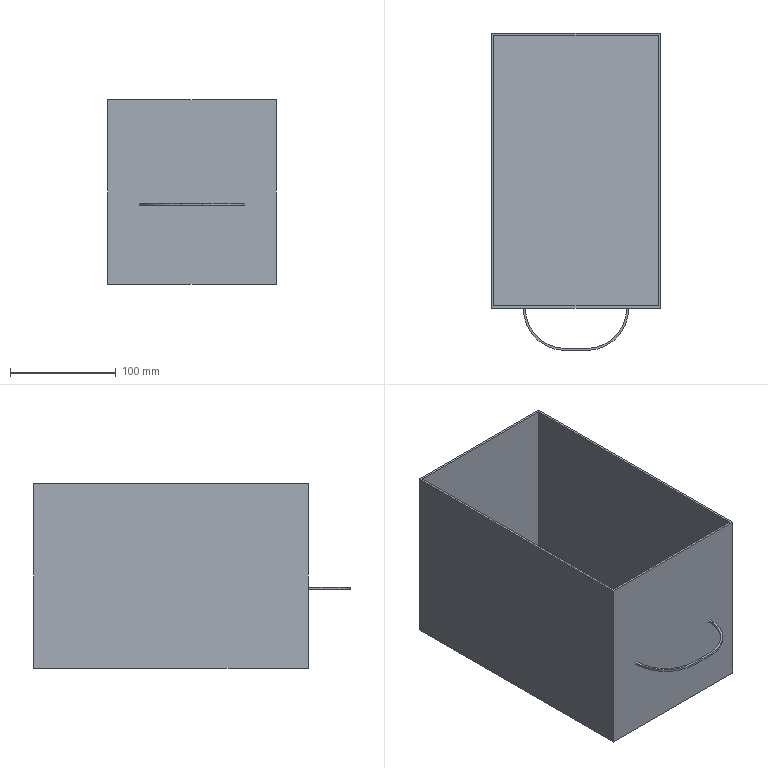Part | NX | features solid 2 | 1 solid | 19 faces | box 160 x 300 x 175 mm | volume 371642 mm3 | plane 15 | cylinder 4 | commonest cylinder face diameters 76 x2 80 x2
STEP:
#1=CARTESIAN_POINT('',(-195.,-510.,-280.));
#2=VERTEX_POINT('',#1);
#3=CARTESIAN_POINT('',(-355.,-510.,-280.));
#4=VERTEX_POINT('',#3);
#5=CARTESIAN_POINT('',(-395.,-510.,-280.));
#6=DIRECTION('',(1.,0.,0.));
#7=VECTOR('',#6,1000.);
#8=LINE('',#5,#7);
#9=EDGE_CURVE('',#2,#4,#8,.F.);
#10=ORIENTED_EDGE('',*,*,#9,.F.);
#11=CARTESIAN_POINT('',(-195.,-510.,-455.));
#12=VERTEX_POINT('',#11);
#13=CARTESIAN_POINT('',(-195.,-510.,-455.));
#14=DIRECTION('',(0.,0.,-1.));
#15=VECTOR('',#14,1000.);
#16=LINE('',#13,#15);
#17=EDGE_CURVE('',#2,#12,#16,.T.);
#18=ORIENTED_EDGE('',*,*,#17,.T.);
#19=CARTESIAN_POINT('',(-355.,-510.,-455.));
#20=VERTEX_POINT('',#19);
#21=CARTESIAN_POINT('',(-395.,-510.,-455.));
#22=DIRECTION('',(1.,0.,0.));
#23=VECTOR('',#22,1000.);
#24=LINE('',#21,#23);
#25=EDGE_CURVE('',#20,#12,#24,.T.);
#26=ORIENTED_EDGE('',*,*,#25,.F.);
#27=CARTESIAN_POINT('',(-355.,-510.,-455.));
#28=DIRECTION('',(0.,0.,1.));
#29=VECTOR('',#28,1000.);
#30=LINE('',#27,#29);
#31=EDGE_CURVE('',#4,#20,#30,.F.);
#32=ORIENTED_EDGE('',*,*,#31,.F.);
#33=EDGE_LOOP('',(#10,#18,#26,#32));
#34=FACE_BOUND('',#33,.T.);
#35=CARTESIAN_POINT('',(-395.,-510.,-455.));
#36=DIRECTION('',(0.,1.,0.));
#37=DIRECTION('',(1.,0.,0.));
#38=AXIS2_PLACEMENT_3D('',#35,#36,#37);
#39=PLANE('',#38);
#40=ADVANCED_FACE('',(#34),#39,.T.);
#41=CARTESIAN_POINT('',(-355.,-770.,-280.));
#42=VERTEX_POINT('',#41);
#43=CARTESIAN_POINT('',(-355.,-510.,-280.));
#44=DIRECTION('',(0.,-1.,0.));
#45=VECTOR('',#44,1000.);
#46=LINE('',#43,#45);
#47=EDGE_CURVE('',#4,#42,#46,.T.);
#48=ORIENTED_EDGE('',*,*,#47,.F.);
#49=ORIENTED_EDGE('',*,*,#31,.T.);
#50=CARTESIAN_POINT('',(-355.,-770.,-455.));
#51=VERTEX_POINT('',#50);
#52=CARTESIAN_POINT('',(-355.,-510.,-455.));
#53=DIRECTION('',(0.,-1.,0.));
#54=VECTOR('',#53,1000.);
#55=LINE('',#52,#54);
#56=EDGE_CURVE('',#20,#51,#55,.T.);
#57=ORIENTED_EDGE('',*,*,#56,.T.);
#58=CARTESIAN_POINT('',(-355.,-770.,-90.));
#59=DIRECTION('',(0.,0.,-1.));
#60=VECTOR('',#59,1000.);
#61=LINE('',#58,#60);
#62=EDGE_CURVE('',#42,#51,#61,.T.);
#63=ORIENTED_EDGE('',*,*,#62,.F.);
#64=EDGE_LOOP('',(#48,#49,#57,#63));
#65=FACE_BOUND('',#64,.T.);
#66=CARTESIAN_POINT('',(-355.,-510.,-455.));
#67=DIRECTION('',(1.,0.,0.));
#68=DIRECTION('',(0.,-1.,0.));
#69=AXIS2_PLACEMENT_3D('',#66,#67,#68);
#70=PLANE('',#69);
#71=ADVANCED_FACE('',(#65),#70,.F.);
#72=CARTESIAN_POINT('',(-227.,-770.,-378.));
#73=VERTEX_POINT('',#72);
#74=CARTESIAN_POINT('',(-225.,-770.,-378.));
#75=VERTEX_POINT('',#74);
#76=CARTESIAN_POINT('',(-315.,-770.,-378.));
#77=DIRECTION('',(-1.,0.,0.));
#78=VECTOR('',#77,1000.);
#79=LINE('',#76,#78);
#80=EDGE_CURVE('',#73,#75,#79,.F.);
#81=ORIENTED_EDGE('',*,*,#80,.T.);
#82=CARTESIAN_POINT('',(-225.,-770.,-380.));
#83=VERTEX_POINT('',#82);
#84=CARTESIAN_POINT('',(-225.,-770.,-380.));
#85=DIRECTION('',(0.,0.,-1.));
#86=VECTOR('',#85,1000.);
#87=LINE('',#84,#86);
#88=EDGE_CURVE('',#75,#83,#87,.T.);
#89=ORIENTED_EDGE('',*,*,#88,.T.);
#90=CARTESIAN_POINT('',(-227.,-770.,-380.));
#91=VERTEX_POINT('',#90);
#92=CARTESIAN_POINT('',(-315.,-770.,-380.));
#93=DIRECTION('',(1.,0.,0.));
#94=VECTOR('',#93,1000.);
#95=LINE('',#92,#94);
#96=EDGE_CURVE('',#91,#83,#95,.T.);
#97=ORIENTED_EDGE('',*,*,#96,.F.);
#98=CARTESIAN_POINT('',(-227.,-770.,-380.));
#99=DIRECTION('',(0.,0.,1.));
#100=VECTOR('',#99,1000.);
#101=LINE('',#98,#100);
#102=EDGE_CURVE('',#73,#91,#101,.F.);
#103=ORIENTED_EDGE('',*,*,#102,.F.);
#104=EDGE_LOOP('',(#81,#89,#97,#103));
#105=FACE_BOUND('',#104,.T.);
#106=CARTESIAN_POINT('',(-325.,-770.,-380.));
#107=VERTEX_POINT('',#106);
#108=CARTESIAN_POINT('',(-323.,-770.,-380.));
#109=VERTEX_POINT('',#108);
#110=CARTESIAN_POINT('',(-315.,-770.,-380.));
#111=DIRECTION('',(1.,0.,0.));
#112=VECTOR('',#111,1000.);
#113=LINE('',#110,#112);
#114=EDGE_CURVE('',#107,#109,#113,.T.);
#115=ORIENTED_EDGE('',*,*,#114,.F.);
#116=CARTESIAN_POINT('',(-325.,-770.,-378.));
#117=VERTEX_POINT('',#116);
#118=CARTESIAN_POINT('',(-325.,-770.,-380.));
#119=DIRECTION('',(0.,0.,1.));
#120=VECTOR('',#119,1000.);
#121=LINE('',#118,#120);
#122=EDGE_CURVE('',#117,#107,#121,.F.);
#123=ORIENTED_EDGE('',*,*,#122,.F.);
#124=CARTESIAN_POINT('',(-323.,-770.,-378.));
#125=VERTEX_POINT('',#124);
#126=CARTESIAN_POINT('',(-315.,-770.,-378.));
#127=DIRECTION('',(-1.,0.,0.));
#128=VECTOR('',#127,1000.);
#129=LINE('',#126,#128);
#130=EDGE_CURVE('',#117,#125,#129,.F.);
#131=ORIENTED_EDGE('',*,*,#130,.T.);
#132=CARTESIAN_POINT('',(-323.,-770.,-380.));
#133=DIRECTION('',(0.,0.,-1.));
#134=VECTOR('',#133,1000.);
#135=LINE('',#132,#134);
#136=EDGE_CURVE('',#125,#109,#135,.T.);
#137=ORIENTED_EDGE('',*,*,#136,.T.);
#138=EDGE_LOOP('',(#115,#123,#131,#137));
#139=FACE_BOUND('',#138,.T.);
#140=CARTESIAN_POINT('',(-195.,-770.,-280.));
#141=VERTEX_POINT('',#140);
#142=CARTESIAN_POINT('',(-17.,-770.,-280.));
#143=DIRECTION('',(1.,0.,0.));
#144=VECTOR('',#143,1000.);
#145=LINE('',#142,#144);
#146=EDGE_CURVE('',#42,#141,#145,.T.);
#147=ORIENTED_EDGE('',*,*,#146,.F.);
#148=ORIENTED_EDGE('',*,*,#62,.T.);
#149=CARTESIAN_POINT('',(-195.,-770.,-455.));
#150=VERTEX_POINT('',#149);
#151=CARTESIAN_POINT('',(-395.,-770.,-455.));
#152=DIRECTION('',(1.,0.,0.));
#153=VECTOR('',#152,1000.);
#154=LINE('',#151,#153);
#155=EDGE_CURVE('',#51,#150,#154,.T.);
#156=ORIENTED_EDGE('',*,*,#155,.T.);
#157=CARTESIAN_POINT('',(-195.,-770.,-455.));
#158=DIRECTION('',(0.,0.,1.));
#159=VECTOR('',#158,1000.);
#160=LINE('',#157,#159);
#161=EDGE_CURVE('',#141,#150,#160,.F.);
#162=ORIENTED_EDGE('',*,*,#161,.F.);
#163=EDGE_LOOP('',(#147,#148,#156,#162));
#164=FACE_BOUND('',#163,.T.);
#165=CARTESIAN_POINT('',(-17.,-770.,-90.));
#166=DIRECTION('',(0.,1.,0.));
#167=DIRECTION('',(0.,0.,1.));
#168=AXIS2_PLACEMENT_3D('',#165,#166,#167);
#169=PLANE('',#168);
#170=ADVANCED_FACE('',(#105,#139,#164),#169,.F.);
#171=CARTESIAN_POINT('',(-195.,-510.,-280.));
#172=DIRECTION('',(0.,-1.,0.));
#173=VECTOR('',#172,1000.);
#174=LINE('',#171,#173);
#175=EDGE_CURVE('',#141,#2,#174,.F.);
#176=ORIENTED_EDGE('',*,*,#175,.F.);
#177=ORIENTED_EDGE('',*,*,#161,.T.);
#178=CARTESIAN_POINT('',(-195.,-510.,-455.));
#179=DIRECTION('',(0.,1.,0.));
#180=VECTOR('',#179,1000.);
#181=LINE('',#178,#180);
#182=EDGE_CURVE('',#12,#150,#181,.F.);
#183=ORIENTED_EDGE('',*,*,#182,.F.);
#184=ORIENTED_EDGE('',*,*,#17,.F.);
#185=EDGE_LOOP('',(#176,#177,#183,#184));
#186=FACE_BOUND('',#185,.T.);
#187=CARTESIAN_POINT('',(-195.,-510.,-455.));
#188=DIRECTION('',(1.,0.,0.));
#189=DIRECTION('',(0.,-1.,0.));
#190=AXIS2_PLACEMENT_3D('',#187,#188,#189);
#191=PLANE('',#190);
#192=ADVANCED_FACE('',(#186),#191,.T.);
#193=ORIENTED_EDGE('',*,*,#155,.F.);
#194=ORIENTED_EDGE('',*,*,#56,.F.);
#195=ORIENTED_EDGE('',*,*,#25,.T.);
#196=ORIENTED_EDGE('',*,*,#182,.T.);
#197=EDGE_LOOP('',(#193,#194,#195,#196));
#198=FACE_BOUND('',#197,.T.);
#199=CARTESIAN_POINT('',(-395.,-510.,-455.));
#200=DIRECTION('',(0.,0.,-1.));
#201=DIRECTION('',(-1.,0.,0.));
#202=AXIS2_PLACEMENT_3D('',#199,#200,#201);
#203=PLANE('',#202);
#204=ADVANCED_FACE('',(#198),#203,.T.);
#205=CARTESIAN_POINT('',(-285.,-808.,-378.));
#206=VERTEX_POINT('',#205);
#207=CARTESIAN_POINT('',(-285.,-770.,-378.));
#208=DIRECTION('',(0.,0.,-1.));
#209=DIRECTION('',(-1.,0.,0.));
#210=AXIS2_PLACEMENT_3D('',#207,#208,#209);
#211=CIRCLE('',#210,38.);
#212=EDGE_CURVE('',#125,#206,#211,.F.);
#213=ORIENTED_EDGE('',*,*,#212,.F.);
#214=ORIENTED_EDGE('',*,*,#130,.F.);
#215=CARTESIAN_POINT('',(-285.,-810.,-378.));
#216=VERTEX_POINT('',#215);
#217=CARTESIAN_POINT('',(-285.,-770.,-378.));
#218=DIRECTION('',(0.,0.,-1.));
#219=DIRECTION('',(-1.,0.,0.));
#220=AXIS2_PLACEMENT_3D('',#217,#218,#219);
#221=CIRCLE('',#220,40.);
#222=EDGE_CURVE('',#117,#216,#221,.F.);
#223=ORIENTED_EDGE('',*,*,#222,.T.);
#224=CARTESIAN_POINT('',(-265.,-810.,-378.));
#225=VERTEX_POINT('',#224);
#226=CARTESIAN_POINT('',(-315.,-810.,-378.));
#227=DIRECTION('',(1.,0.,0.));
#228=VECTOR('',#227,1000.);
#229=LINE('',#226,#228);
#230=EDGE_CURVE('',#216,#225,#229,.T.);
#231=ORIENTED_EDGE('',*,*,#230,.T.);
#232=CARTESIAN_POINT('',(-265.,-770.,-378.));
#233=DIRECTION('',(0.,0.,-1.));
#234=DIRECTION('',(-1.,0.,0.));
#235=AXIS2_PLACEMENT_3D('',#232,#233,#234);
#236=CIRCLE('',#235,40.);
#237=EDGE_CURVE('',#225,#75,#236,.F.);
#238=ORIENTED_EDGE('',*,*,#237,.T.);
#239=ORIENTED_EDGE('',*,*,#80,.F.);
#240=CARTESIAN_POINT('',(-265.,-808.,-378.));
#241=VERTEX_POINT('',#240);
#242=CARTESIAN_POINT('',(-265.,-770.,-378.));
#243=DIRECTION('',(0.,0.,-1.));
#244=DIRECTION('',(-1.,0.,0.));
#245=AXIS2_PLACEMENT_3D('',#242,#243,#244);
#246=CIRCLE('',#245,38.);
#247=EDGE_CURVE('',#241,#73,#246,.F.);
#248=ORIENTED_EDGE('',*,*,#247,.F.);
#249=CARTESIAN_POINT('',(-315.,-808.,-378.));
#250=DIRECTION('',(1.,0.,0.));
#251=VECTOR('',#250,1000.);
#252=LINE('',#249,#251);
#253=EDGE_CURVE('',#206,#241,#252,.T.);
#254=ORIENTED_EDGE('',*,*,#253,.F.);
#255=EDGE_LOOP('',(#213,#214,#223,#231,#238,#239,#248,#254));
#256=FACE_BOUND('',#255,.T.);
#257=CARTESIAN_POINT('',(-315.,-770.,-378.));
#258=DIRECTION('',(0.,0.,-1.));
#259=DIRECTION('',(-1.,0.,0.));
#260=AXIS2_PLACEMENT_3D('',#257,#258,#259);
#261=PLANE('',#260);
#262=ADVANCED_FACE('',(#256),#261,.F.);
#263=ORIENTED_EDGE('',*,*,#230,.F.);
#264=CARTESIAN_POINT('',(-285.,-810.,-380.));
#265=VERTEX_POINT('',#264);
#266=CARTESIAN_POINT('',(-285.,-810.,-380.));
#267=DIRECTION('',(0.,0.,-1.));
#268=VECTOR('',#267,1000.);
#269=LINE('',#266,#268);
#270=EDGE_CURVE('',#216,#265,#269,.T.);
#271=ORIENTED_EDGE('',*,*,#270,.T.);
#272=CARTESIAN_POINT('',(-265.,-810.,-380.));
#273=VERTEX_POINT('',#272);
#274=CARTESIAN_POINT('',(-315.,-810.,-380.));
#275=DIRECTION('',(1.,0.,0.));
#276=VECTOR('',#275,1000.);
#277=LINE('',#274,#276);
#278=EDGE_CURVE('',#265,#273,#277,.T.);
#279=ORIENTED_EDGE('',*,*,#278,.T.);
#280=CARTESIAN_POINT('',(-265.,-810.,-380.));
#281=DIRECTION('',(0.,0.,1.));
#282=VECTOR('',#281,1000.);
#283=LINE('',#280,#282);
#284=EDGE_CURVE('',#273,#225,#283,.T.);
#285=ORIENTED_EDGE('',*,*,#284,.T.);
#286=EDGE_LOOP('',(#263,#271,#279,#285));
#287=FACE_BOUND('',#286,.T.);
#288=CARTESIAN_POINT('',(-315.,-810.,-380.));
#289=DIRECTION('',(0.,1.,0.));
#290=DIRECTION('',(1.,0.,0.));
#291=AXIS2_PLACEMENT_3D('',#288,#289,#290);
#292=PLANE('',#291);
#293=ADVANCED_FACE('',(#287),#292,.F.);
#294=CARTESIAN_POINT('',(-285.,-808.,-380.));
#295=VERTEX_POINT('',#294);
#296=CARTESIAN_POINT('',(-285.,-770.,-380.));
#297=DIRECTION('',(0.,0.,-1.));
#298=DIRECTION('',(-1.,0.,0.));
#299=AXIS2_PLACEMENT_3D('',#296,#297,#298);
#300=CIRCLE('',#299,38.);
#301=EDGE_CURVE('',#295,#109,#300,.T.);
#302=ORIENTED_EDGE('',*,*,#301,.F.);
#303=CARTESIAN_POINT('',(-265.,-808.,-380.));
#304=VERTEX_POINT('',#303);
#305=CARTESIAN_POINT('',(-315.,-808.,-380.));
#306=DIRECTION('',(1.,0.,0.));
#307=VECTOR('',#306,1000.);
#308=LINE('',#305,#307);
#309=EDGE_CURVE('',#295,#304,#308,.T.);
#310=ORIENTED_EDGE('',*,*,#309,.T.);
#311=CARTESIAN_POINT('',(-265.,-770.,-380.));
#312=DIRECTION('',(0.,0.,-1.));
#313=DIRECTION('',(-1.,0.,0.));
#314=AXIS2_PLACEMENT_3D('',#311,#312,#313);
#315=CIRCLE('',#314,38.);
#316=EDGE_CURVE('',#91,#304,#315,.T.);
#317=ORIENTED_EDGE('',*,*,#316,.F.);
#318=ORIENTED_EDGE('',*,*,#96,.T.);
#319=CARTESIAN_POINT('',(-265.,-770.,-380.));
#320=DIRECTION('',(0.,0.,-1.));
#321=DIRECTION('',(-1.,0.,0.));
#322=AXIS2_PLACEMENT_3D('',#319,#320,#321);
#323=CIRCLE('',#322,40.);
#324=EDGE_CURVE('',#83,#273,#323,.T.);
#325=ORIENTED_EDGE('',*,*,#324,.T.);
#326=ORIENTED_EDGE('',*,*,#278,.F.);
#327=CARTESIAN_POINT('',(-285.,-770.,-380.));
#328=DIRECTION('',(0.,0.,-1.));
#329=DIRECTION('',(-1.,0.,0.));
#330=AXIS2_PLACEMENT_3D('',#327,#328,#329);
#331=CIRCLE('',#330,40.);
#332=EDGE_CURVE('',#265,#107,#331,.T.);
#333=ORIENTED_EDGE('',*,*,#332,.T.);
#334=ORIENTED_EDGE('',*,*,#114,.T.);
#335=EDGE_LOOP('',(#302,#310,#317,#318,#325,#326,#333,#334));
#336=FACE_BOUND('',#335,.T.);
#337=CARTESIAN_POINT('',(-315.,-770.,-380.));
#338=DIRECTION('',(0.,0.,-1.));
#339=DIRECTION('',(-1.,0.,0.));
#340=AXIS2_PLACEMENT_3D('',#337,#338,#339);
#341=PLANE('',#340);
#342=ADVANCED_FACE('',(#336),#341,.T.);
#343=ORIENTED_EDGE('',*,*,#222,.F.);
#344=ORIENTED_EDGE('',*,*,#122,.T.);
#345=ORIENTED_EDGE('',*,*,#332,.F.);
#346=ORIENTED_EDGE('',*,*,#270,.F.);
#347=EDGE_LOOP('',(#343,#344,#345,#346));
#348=FACE_BOUND('',#347,.T.);
#349=CARTESIAN_POINT('',(-285.,-770.,-380.));
#350=DIRECTION('',(0.,0.,-1.));
#351=DIRECTION('',(-1.,0.,0.));
#352=AXIS2_PLACEMENT_3D('',#349,#350,#351);
#353=CYLINDRICAL_SURFACE('',#352,40.);
#354=ADVANCED_FACE('',(#348),#353,.T.);
#355=ORIENTED_EDGE('',*,*,#237,.F.);
#356=ORIENTED_EDGE('',*,*,#284,.F.);
#357=ORIENTED_EDGE('',*,*,#324,.F.);
#358=ORIENTED_EDGE('',*,*,#88,.F.);
#359=EDGE_LOOP('',(#355,#356,#357,#358));
#360=FACE_BOUND('',#359,.T.);
#361=CARTESIAN_POINT('',(-265.,-770.,-380.));
#362=DIRECTION('',(0.,0.,1.));
#363=DIRECTION('',(1.,0.,0.));
#364=AXIS2_PLACEMENT_3D('',#361,#362,#363);
#365=CYLINDRICAL_SURFACE('',#364,40.);
#366=ADVANCED_FACE('',(#360),#365,.T.);
#367=ORIENTED_EDGE('',*,*,#253,.T.);
#368=CARTESIAN_POINT('',(-265.,-808.,-380.));
#369=DIRECTION('',(0.,0.,-1.));
#370=VECTOR('',#369,1000.);
#371=LINE('',#368,#370);
#372=EDGE_CURVE('',#304,#241,#371,.F.);
#373=ORIENTED_EDGE('',*,*,#372,.F.);
#374=ORIENTED_EDGE('',*,*,#309,.F.);
#375=CARTESIAN_POINT('',(-285.,-808.,-380.));
#376=DIRECTION('',(0.,0.,-1.));
#377=VECTOR('',#376,1000.);
#378=LINE('',#375,#377);
#379=EDGE_CURVE('',#206,#295,#378,.T.);
#380=ORIENTED_EDGE('',*,*,#379,.F.);
#381=EDGE_LOOP('',(#367,#373,#374,#380));
#382=FACE_BOUND('',#381,.T.);
#383=CARTESIAN_POINT('',(-315.,-808.,-380.));
#384=DIRECTION('',(0.,1.,0.));
#385=DIRECTION('',(1.,0.,0.));
#386=AXIS2_PLACEMENT_3D('',#383,#384,#385);
#387=PLANE('',#386);
#388=ADVANCED_FACE('',(#382),#387,.T.);
#389=ORIENTED_EDGE('',*,*,#212,.T.);
#390=ORIENTED_EDGE('',*,*,#379,.T.);
#391=ORIENTED_EDGE('',*,*,#301,.T.);
#392=ORIENTED_EDGE('',*,*,#136,.F.);
#393=EDGE_LOOP('',(#389,#390,#391,#392));
#394=FACE_BOUND('',#393,.T.);
#395=CARTESIAN_POINT('',(-285.,-770.,-380.));
#396=DIRECTION('',(0.,0.,-1.));
#397=DIRECTION('',(-1.,0.,0.));
#398=AXIS2_PLACEMENT_3D('',#395,#396,#397);
#399=CYLINDRICAL_SURFACE('',#398,38.);
#400=ADVANCED_FACE('',(#394),#399,.F.);
#401=ORIENTED_EDGE('',*,*,#247,.T.);
#402=ORIENTED_EDGE('',*,*,#102,.T.);
#403=ORIENTED_EDGE('',*,*,#316,.T.);
#404=ORIENTED_EDGE('',*,*,#372,.T.);
#405=EDGE_LOOP('',(#401,#402,#403,#404));
#406=FACE_BOUND('',#405,.T.);
#407=CARTESIAN_POINT('',(-265.,-770.,-380.));
#408=DIRECTION('',(0.,0.,1.));
#409=DIRECTION('',(1.,0.,0.));
#410=AXIS2_PLACEMENT_3D('',#407,#408,#409);
#411=CYLINDRICAL_SURFACE('',#410,38.);
#412=ADVANCED_FACE('',(#406),#411,.F.);
#413=CARTESIAN_POINT('',(-197.,-512.,-280.));
#414=VERTEX_POINT('',#413);
#415=CARTESIAN_POINT('',(-353.,-512.,-280.));
#416=VERTEX_POINT('',#415);
#417=CARTESIAN_POINT('',(-395.,-512.,-280.));
#418=DIRECTION('',(1.,0.,0.));
#419=VECTOR('',#418,1000.);
#420=LINE('',#417,#419);
#421=EDGE_CURVE('',#414,#416,#420,.F.);
#422=ORIENTED_EDGE('',*,*,#421,.F.);
#423=CARTESIAN_POINT('',(-197.,-768.,-280.));
#424=VERTEX_POINT('',#423);
#425=CARTESIAN_POINT('',(-197.,-510.,-280.));
#426=DIRECTION('',(0.,-1.,0.));
#427=VECTOR('',#426,1000.);
#428=LINE('',#425,#427);
#429=EDGE_CURVE('',#424,#414,#428,.F.);
#430=ORIENTED_EDGE('',*,*,#429,.F.);
#431=CARTESIAN_POINT('',(-353.,-768.,-280.));
#432=VERTEX_POINT('',#431);
#433=CARTESIAN_POINT('',(-17.,-768.,-280.));
#434=DIRECTION('',(1.,0.,0.));
#435=VECTOR('',#434,1000.);
#436=LINE('',#433,#435);
#437=EDGE_CURVE('',#432,#424,#436,.T.);
#438=ORIENTED_EDGE('',*,*,#437,.F.);
#439=CARTESIAN_POINT('',(-353.,-510.,-280.));
#440=DIRECTION('',(0.,-1.,0.));
#441=VECTOR('',#440,1000.);
#442=LINE('',#439,#441);
#443=EDGE_CURVE('',#416,#432,#442,.T.);
#444=ORIENTED_EDGE('',*,*,#443,.F.);
#445=EDGE_LOOP('',(#422,#430,#438,#444));
#446=FACE_BOUND('',#445,.T.);
#447=ORIENTED_EDGE('',*,*,#175,.T.);
#448=ORIENTED_EDGE('',*,*,#9,.T.);
#449=ORIENTED_EDGE('',*,*,#47,.T.);
#450=ORIENTED_EDGE('',*,*,#146,.T.);
#451=EDGE_LOOP('',(#447,#448,#449,#450));
#452=FACE_BOUND('',#451,.T.);
#453=CARTESIAN_POINT('',(-275.,-640.,-280.));
#454=DIRECTION('',(0.,0.,1.));
#455=DIRECTION('',(1.,0.,0.));
#456=AXIS2_PLACEMENT_3D('',#453,#454,#455);
#457=PLANE('',#456);
#458=ADVANCED_FACE('',(#446,#452),#457,.T.);
#459=CARTESIAN_POINT('',(-353.,-768.,-453.));
#460=VERTEX_POINT('',#459);
#461=CARTESIAN_POINT('',(-197.,-768.,-453.));
#462=VERTEX_POINT('',#461);
#463=CARTESIAN_POINT('',(-395.,-768.,-453.));
#464=DIRECTION('',(1.,0.,0.));
#465=VECTOR('',#464,1000.);
#466=LINE('',#463,#465);
#467=EDGE_CURVE('',#460,#462,#466,.T.);
#468=ORIENTED_EDGE('',*,*,#467,.T.);
#469=CARTESIAN_POINT('',(-197.,-512.,-453.));
#470=VERTEX_POINT('',#469);
#471=CARTESIAN_POINT('',(-197.,-510.,-453.));
#472=DIRECTION('',(0.,1.,0.));
#473=VECTOR('',#472,1000.);
#474=LINE('',#471,#473);
#475=EDGE_CURVE('',#470,#462,#474,.F.);
#476=ORIENTED_EDGE('',*,*,#475,.F.);
#477=CARTESIAN_POINT('',(-353.,-512.,-453.));
#478=VERTEX_POINT('',#477);
#479=CARTESIAN_POINT('',(-395.,-512.,-453.));
#480=DIRECTION('',(-1.,0.,0.));
#481=VECTOR('',#480,1000.);
#482=LINE('',#479,#481);
#483=EDGE_CURVE('',#478,#470,#482,.F.);
#484=ORIENTED_EDGE('',*,*,#483,.F.);
#485=CARTESIAN_POINT('',(-353.,-510.,-453.));
#486=DIRECTION('',(0.,-1.,0.));
#487=VECTOR('',#486,1000.);
#488=LINE('',#485,#487);
#489=EDGE_CURVE('',#478,#460,#488,.T.);
#490=ORIENTED_EDGE('',*,*,#489,.T.);
#491=EDGE_LOOP('',(#468,#476,#484,#490));
#492=FACE_BOUND('',#491,.T.);
#493=CARTESIAN_POINT('',(-395.,-510.,-453.));
#494=DIRECTION('',(0.,0.,-1.));
#495=DIRECTION('',(-1.,0.,0.));
#496=AXIS2_PLACEMENT_3D('',#493,#494,#495);
#497=PLANE('',#496);
#498=ADVANCED_FACE('',(#492),#497,.F.);
#499=CARTESIAN_POINT('',(-197.,-768.,-455.));
#500=DIRECTION('',(0.,0.,1.));
#501=VECTOR('',#500,1000.);
#502=LINE('',#499,#501);
#503=EDGE_CURVE('',#424,#462,#502,.F.);
#504=ORIENTED_EDGE('',*,*,#503,.F.);
#505=ORIENTED_EDGE('',*,*,#429,.T.);
#506=CARTESIAN_POINT('',(-197.,-512.,-455.));
#507=DIRECTION('',(0.,0.,-1.));
#508=VECTOR('',#507,1000.);
#509=LINE('',#506,#508);
#510=EDGE_CURVE('',#414,#470,#509,.T.);
#511=ORIENTED_EDGE('',*,*,#510,.T.);
#512=ORIENTED_EDGE('',*,*,#475,.T.);
#513=EDGE_LOOP('',(#504,#505,#511,#512));
#514=FACE_BOUND('',#513,.T.);
#515=CARTESIAN_POINT('',(-197.,-510.,-455.));
#516=DIRECTION('',(1.,0.,0.));
#517=DIRECTION('',(0.,-1.,0.));
#518=AXIS2_PLACEMENT_3D('',#515,#516,#517);
#519=PLANE('',#518);
#520=ADVANCED_FACE('',(#514),#519,.F.);
#521=CARTESIAN_POINT('',(-353.,-768.,-90.));
#522=DIRECTION('',(0.,0.,-1.));
#523=VECTOR('',#522,1000.);
#524=LINE('',#521,#523);
#525=EDGE_CURVE('',#432,#460,#524,.T.);
#526=ORIENTED_EDGE('',*,*,#525,.F.);
#527=ORIENTED_EDGE('',*,*,#437,.T.);
#528=ORIENTED_EDGE('',*,*,#503,.T.);
#529=ORIENTED_EDGE('',*,*,#467,.F.);
#530=EDGE_LOOP('',(#526,#527,#528,#529));
#531=FACE_BOUND('',#530,.T.);
#532=CARTESIAN_POINT('',(-17.,-768.,-90.));
#533=DIRECTION('',(0.,1.,0.));
#534=DIRECTION('',(0.,0.,1.));
#535=AXIS2_PLACEMENT_3D('',#532,#533,#534);
#536=PLANE('',#535);
#537=ADVANCED_FACE('',(#531),#536,.T.);
#538=CARTESIAN_POINT('',(-353.,-512.,-455.));
#539=DIRECTION('',(0.,0.,1.));
#540=VECTOR('',#539,1000.);
#541=LINE('',#538,#540);
#542=EDGE_CURVE('',#416,#478,#541,.F.);
#543=ORIENTED_EDGE('',*,*,#542,.F.);
#544=ORIENTED_EDGE('',*,*,#443,.T.);
#545=ORIENTED_EDGE('',*,*,#525,.T.);
#546=ORIENTED_EDGE('',*,*,#489,.F.);
#547=EDGE_LOOP('',(#543,#544,#545,#546));
#548=FACE_BOUND('',#547,.T.);
#549=CARTESIAN_POINT('',(-353.,-510.,-455.));
#550=DIRECTION('',(1.,0.,0.));
#551=DIRECTION('',(0.,-1.,0.));
#552=AXIS2_PLACEMENT_3D('',#549,#550,#551);
#553=PLANE('',#552);
#554=ADVANCED_FACE('',(#548),#553,.T.);
#555=ORIENTED_EDGE('',*,*,#510,.F.);
#556=ORIENTED_EDGE('',*,*,#421,.T.);
#557=ORIENTED_EDGE('',*,*,#542,.T.);
#558=ORIENTED_EDGE('',*,*,#483,.T.);
#559=EDGE_LOOP('',(#555,#556,#557,#558));
#560=FACE_BOUND('',#559,.T.);
#561=CARTESIAN_POINT('',(-395.,-512.,-455.));
#562=DIRECTION('',(0.,1.,0.));
#563=DIRECTION('',(1.,0.,0.));
#564=AXIS2_PLACEMENT_3D('',#561,#562,#563);
#565=PLANE('',#564);
#566=ADVANCED_FACE('',(#560),#565,.F.);
#567=CLOSED_SHELL('',(#40,#71,#170,#192,#204,#262,#293,#342,#354,#366,#388,#400,#412,#458,#498,#520,#537,#554,#566));
#568=MANIFOLD_SOLID_BREP('',#567);
#569=(LENGTH_UNIT()NAMED_UNIT(*)SI_UNIT(.MILLI.,.METRE.));
#570=UNCERTAINTY_MEASURE_WITH_UNIT(LENGTH_MEASURE(0.00001),#569,'','');
#571=(NAMED_UNIT(*)PLANE_ANGLE_UNIT()SI_UNIT($,.RADIAN.));
#572=(NAMED_UNIT(*)SI_UNIT($,.STERADIAN.)SOLID_ANGLE_UNIT());
#573=(GEOMETRIC_REPRESENTATION_CONTEXT(3)GLOBAL_UNCERTAINTY_ASSIGNED_CONTEXT((#570))GLOBAL_UNIT_ASSIGNED_CONTEXT((#569,#571,#572))REPRESENTATION_CONTEXT('',''));
#574=ADVANCED_BREP_SHAPE_REPRESENTATION('',(#568),#573);